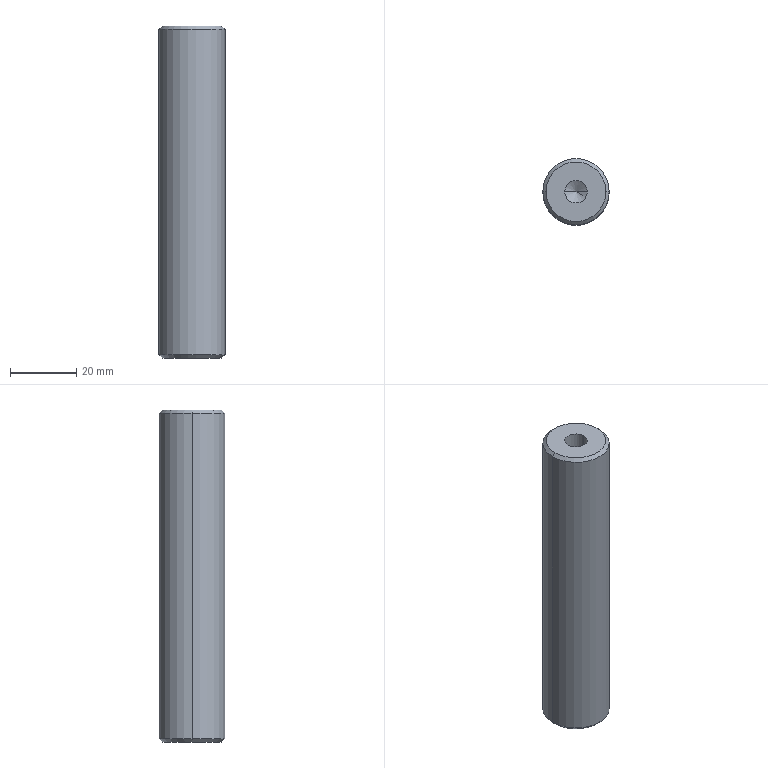Part | SolidWorks | features Chamfer 2, HoleWzd 2, Extrusion 1 | 1 solid | 16 faces | box 20 x 20 x 100 mm | volume 29690 mm3 | cone 8 | cylinder 6 | plane 2 | commonest cylinder face diameters 6.8 x4 20 x2
STEP:
#1=CARTESIAN_POINT('',(3.4,0.,22.25));
#2=VERTEX_POINT('',#1);
#3=CARTESIAN_POINT('',(-3.4,0.,22.25));
#4=VERTEX_POINT('',#3);
#5=CARTESIAN_POINT('',(0.,0.,22.25));
#6=DIRECTION('',(0.,0.,-1.));
#7=DIRECTION('',(-1.,0.,0.));
#8=AXIS2_PLACEMENT_3D('',#5,#6,#7);
#9=CIRCLE('',#8,3.4);
#10=EDGE_CURVE('',#2,#4,#9,.T.);
#11=ORIENTED_EDGE('',*,*,#10,.F.);
#12=CARTESIAN_POINT('',(3.4,0.,0.));
#13=VERTEX_POINT('',#12);
#14=CARTESIAN_POINT('',(3.4,0.,0.));
#15=DIRECTION('',(0.,0.,-1.));
#16=VECTOR('',#15,1000.);
#17=LINE('',#14,#16);
#18=EDGE_CURVE('',#2,#13,#17,.T.);
#19=ORIENTED_EDGE('',*,*,#18,.T.);
#20=CARTESIAN_POINT('',(-3.4,0.,0.));
#21=VERTEX_POINT('',#20);
#22=CARTESIAN_POINT('',(0.,0.,0.));
#23=DIRECTION('',(0.,0.,-1.));
#24=DIRECTION('',(-1.,0.,0.));
#25=AXIS2_PLACEMENT_3D('',#22,#23,#24);
#26=CIRCLE('',#25,3.4);
#27=EDGE_CURVE('',#13,#21,#26,.T.);
#28=ORIENTED_EDGE('',*,*,#27,.T.);
#29=CARTESIAN_POINT('',(-3.4,0.,0.));
#30=DIRECTION('',(0.,0.,-1.));
#31=VECTOR('',#30,1000.);
#32=LINE('',#29,#31);
#33=EDGE_CURVE('',#4,#21,#32,.T.);
#34=ORIENTED_EDGE('',*,*,#33,.F.);
#35=EDGE_LOOP('',(#11,#19,#28,#34));
#36=FACE_OUTER_BOUND('',#35,.T.);
#37=CARTESIAN_POINT('',(0.,0.,0.));
#38=DIRECTION('',(0.,0.,-1.));
#39=DIRECTION('',(-1.,0.,0.));
#40=AXIS2_PLACEMENT_3D('',#37,#38,#39);
#41=CYLINDRICAL_SURFACE('',#40,3.4);
#42=ADVANCED_FACE('',(#36),#41,.F.);
#43=CARTESIAN_POINT('',(0.,0.,24.293));
#44=VERTEX_POINT('',#43);
#45=CARTESIAN_POINT('',(-3.4,0.,22.25));
#46=DIRECTION('',(-0.8572,0.,-0.515));
#47=VECTOR('',#46,1000.);
#48=LINE('',#45,#47);
#49=EDGE_CURVE('',#44,#4,#48,.T.);
#50=ORIENTED_EDGE('',*,*,#49,.F.);
#51=CARTESIAN_POINT('',(3.4,0.,22.25));
#52=DIRECTION('',(0.8572,0.,-0.515));
#53=VECTOR('',#52,1000.);
#54=LINE('',#51,#53);
#55=EDGE_CURVE('',#44,#2,#54,.T.);
#56=ORIENTED_EDGE('',*,*,#55,.T.);
#57=ORIENTED_EDGE('',*,*,#10,.T.);
#58=EDGE_LOOP('',(#50,#56,#57));
#59=FACE_OUTER_BOUND('',#58,.T.);
#60=CARTESIAN_POINT('',(0.,0.,22.25));
#61=DIRECTION('',(0.,0.,-1.));
#62=DIRECTION('',(-1.,0.,0.));
#63=AXIS2_PLACEMENT_3D('',#60,#61,#62);
#64=CONICAL_SURFACE('',#63,3.4,1.03);
#65=ADVANCED_FACE('',(#59),#64,.F.);
#66=CARTESIAN_POINT('',(-9.,0.,0.));
#67=VERTEX_POINT('',#66);
#68=CARTESIAN_POINT('',(9.,0.,0.));
#69=VERTEX_POINT('',#68);
#70=CARTESIAN_POINT('',(0.,0.,0.));
#71=DIRECTION('',(0.,0.,-1.));
#72=DIRECTION('',(1.,0.,0.));
#73=AXIS2_PLACEMENT_3D('',#70,#71,#72);
#74=CIRCLE('',#73,9.);
#75=EDGE_CURVE('',#67,#69,#74,.T.);
#76=ORIENTED_EDGE('',*,*,#75,.F.);
#77=CARTESIAN_POINT('',(-10.,0.,1.));
#78=VERTEX_POINT('',#77);
#79=CARTESIAN_POINT('',(-10.,0.,1.));
#80=DIRECTION('',(-0.7071,0.,0.7071));
#81=VECTOR('',#80,1000.);
#82=LINE('',#79,#81);
#83=EDGE_CURVE('',#67,#78,#82,.T.);
#84=ORIENTED_EDGE('',*,*,#83,.T.);
#85=CARTESIAN_POINT('',(10.,0.,1.));
#86=VERTEX_POINT('',#85);
#87=CARTESIAN_POINT('',(0.,0.,1.));
#88=DIRECTION('',(0.,0.,1.));
#89=DIRECTION('',(1.,0.,0.));
#90=AXIS2_PLACEMENT_3D('',#87,#88,#89);
#91=CIRCLE('',#90,10.);
#92=EDGE_CURVE('',#86,#78,#91,.T.);
#93=ORIENTED_EDGE('',*,*,#92,.F.);
#94=CARTESIAN_POINT('',(10.,0.,1.));
#95=DIRECTION('',(0.7071,0.,0.7071));
#96=VECTOR('',#95,1000.);
#97=LINE('',#94,#96);
#98=EDGE_CURVE('',#69,#86,#97,.T.);
#99=ORIENTED_EDGE('',*,*,#98,.F.);
#100=EDGE_LOOP('',(#76,#84,#93,#99));
#101=FACE_OUTER_BOUND('',#100,.T.);
#102=CARTESIAN_POINT('',(0.,0.,1.));
#103=DIRECTION('',(0.,0.,1.));
#104=DIRECTION('',(1.,0.,0.));
#105=AXIS2_PLACEMENT_3D('',#102,#103,#104);
#106=CONICAL_SURFACE('',#105,10.,0.7854);
#107=ADVANCED_FACE('',(#101),#106,.T.);
#108=CARTESIAN_POINT('',(9.,0.,100.));
#109=VERTEX_POINT('',#108);
#110=CARTESIAN_POINT('',(-9.,0.,100.));
#111=VERTEX_POINT('',#110);
#112=CARTESIAN_POINT('',(0.,0.,100.));
#113=DIRECTION('',(0.,0.,1.));
#114=DIRECTION('',(1.,0.,0.));
#115=AXIS2_PLACEMENT_3D('',#112,#113,#114);
#116=CIRCLE('',#115,9.);
#117=EDGE_CURVE('',#109,#111,#116,.T.);
#118=ORIENTED_EDGE('',*,*,#117,.F.);
#119=CARTESIAN_POINT('',(10.,0.,99.));
#120=VERTEX_POINT('',#119);
#121=CARTESIAN_POINT('',(9.,0.,100.));
#122=DIRECTION('',(0.7071,0.,-0.7071));
#123=VECTOR('',#122,1000.);
#124=LINE('',#121,#123);
#125=EDGE_CURVE('',#109,#120,#124,.T.);
#126=ORIENTED_EDGE('',*,*,#125,.T.);
#127=CARTESIAN_POINT('',(-10.,0.,99.));
#128=VERTEX_POINT('',#127);
#129=CARTESIAN_POINT('',(0.,0.,99.));
#130=DIRECTION('',(0.,0.,-1.));
#131=DIRECTION('',(1.,0.,0.));
#132=AXIS2_PLACEMENT_3D('',#129,#130,#131);
#133=CIRCLE('',#132,10.);
#134=EDGE_CURVE('',#128,#120,#133,.T.);
#135=ORIENTED_EDGE('',*,*,#134,.F.);
#136=CARTESIAN_POINT('',(-9.,0.,100.));
#137=DIRECTION('',(-0.7071,0.,-0.7071));
#138=VECTOR('',#137,1000.);
#139=LINE('',#136,#138);
#140=EDGE_CURVE('',#111,#128,#139,.T.);
#141=ORIENTED_EDGE('',*,*,#140,.F.);
#142=EDGE_LOOP('',(#118,#126,#135,#141));
#143=FACE_OUTER_BOUND('',#142,.T.);
#144=CARTESIAN_POINT('',(0.,0.,100.));
#145=DIRECTION('',(0.,0.,-1.));
#146=DIRECTION('',(-1.,0.,0.));
#147=AXIS2_PLACEMENT_3D('',#144,#145,#146);
#148=CONICAL_SURFACE('',#147,9.,0.7854);
#149=ADVANCED_FACE('',(#143),#148,.T.);
#150=CARTESIAN_POINT('',(-3.4,0.,77.75));
#151=VERTEX_POINT('',#150);
#152=CARTESIAN_POINT('',(3.4,0.,77.75));
#153=VERTEX_POINT('',#152);
#154=CARTESIAN_POINT('',(0.,0.,77.75));
#155=DIRECTION('',(0.,0.,1.));
#156=DIRECTION('',(1.,0.,0.));
#157=AXIS2_PLACEMENT_3D('',#154,#155,#156);
#158=CIRCLE('',#157,3.4);
#159=EDGE_CURVE('',#151,#153,#158,.T.);
#160=ORIENTED_EDGE('',*,*,#159,.F.);
#161=CARTESIAN_POINT('',(-3.4,0.,100.));
#162=VERTEX_POINT('',#161);
#163=CARTESIAN_POINT('',(-3.4,0.,100.));
#164=DIRECTION('',(0.,0.,1.));
#165=VECTOR('',#164,1000.);
#166=LINE('',#163,#165);
#167=EDGE_CURVE('',#151,#162,#166,.T.);
#168=ORIENTED_EDGE('',*,*,#167,.T.);
#169=CARTESIAN_POINT('',(3.4,0.,100.));
#170=VERTEX_POINT('',#169);
#171=CARTESIAN_POINT('',(0.,0.,100.));
#172=DIRECTION('',(0.,0.,1.));
#173=DIRECTION('',(1.,0.,0.));
#174=AXIS2_PLACEMENT_3D('',#171,#172,#173);
#175=CIRCLE('',#174,3.4);
#176=EDGE_CURVE('',#162,#170,#175,.T.);
#177=ORIENTED_EDGE('',*,*,#176,.T.);
#178=CARTESIAN_POINT('',(3.4,0.,100.));
#179=DIRECTION('',(0.,0.,1.));
#180=VECTOR('',#179,1000.);
#181=LINE('',#178,#180);
#182=EDGE_CURVE('',#153,#170,#181,.T.);
#183=ORIENTED_EDGE('',*,*,#182,.F.);
#184=EDGE_LOOP('',(#160,#168,#177,#183));
#185=FACE_OUTER_BOUND('',#184,.T.);
#186=CARTESIAN_POINT('',(0.,0.,100.));
#187=DIRECTION('',(0.,0.,1.));
#188=DIRECTION('',(1.,0.,0.));
#189=AXIS2_PLACEMENT_3D('',#186,#187,#188);
#190=CYLINDRICAL_SURFACE('',#189,3.4);
#191=ADVANCED_FACE('',(#185),#190,.F.);
#192=CARTESIAN_POINT('',(0.,0.,75.707));
#193=VERTEX_POINT('',#192);
#194=CARTESIAN_POINT('',(3.4,0.,77.75));
#195=DIRECTION('',(0.8572,0.,0.515));
#196=VECTOR('',#195,1000.);
#197=LINE('',#194,#196);
#198=EDGE_CURVE('',#193,#153,#197,.T.);
#199=ORIENTED_EDGE('',*,*,#198,.F.);
#200=CARTESIAN_POINT('',(-3.4,0.,77.75));
#201=DIRECTION('',(-0.8572,0.,0.515));
#202=VECTOR('',#201,1000.);
#203=LINE('',#200,#202);
#204=EDGE_CURVE('',#193,#151,#203,.T.);
#205=ORIENTED_EDGE('',*,*,#204,.T.);
#206=ORIENTED_EDGE('',*,*,#159,.T.);
#207=EDGE_LOOP('',(#199,#205,#206));
#208=FACE_OUTER_BOUND('',#207,.T.);
#209=CARTESIAN_POINT('',(0.,0.,77.75));
#210=DIRECTION('',(0.,0.,1.));
#211=DIRECTION('',(1.,0.,0.));
#212=AXIS2_PLACEMENT_3D('',#209,#210,#211);
#213=CONICAL_SURFACE('',#212,3.4,1.03);
#214=ADVANCED_FACE('',(#208),#213,.F.);
#215=ORIENTED_EDGE('',*,*,#134,.T.);
#216=CARTESIAN_POINT('',(10.,0.,100.));
#217=DIRECTION('',(0.,0.,-1.));
#218=VECTOR('',#217,1000.);
#219=LINE('',#216,#218);
#220=EDGE_CURVE('',#120,#86,#219,.T.);
#221=ORIENTED_EDGE('',*,*,#220,.T.);
#222=ORIENTED_EDGE('',*,*,#92,.T.);
#223=CARTESIAN_POINT('',(-10.,0.,100.));
#224=DIRECTION('',(0.,0.,-1.));
#225=VECTOR('',#224,1000.);
#226=LINE('',#223,#225);
#227=EDGE_CURVE('',#128,#78,#226,.T.);
#228=ORIENTED_EDGE('',*,*,#227,.F.);
#229=EDGE_LOOP('',(#215,#221,#222,#228));
#230=FACE_OUTER_BOUND('',#229,.T.);
#231=CARTESIAN_POINT('',(0.,0.,100.));
#232=DIRECTION('',(0.,0.,-1.));
#233=DIRECTION('',(-1.,0.,0.));
#234=AXIS2_PLACEMENT_3D('',#231,#232,#233);
#235=CYLINDRICAL_SURFACE('',#234,10.);
#236=ADVANCED_FACE('',(#230),#235,.T.);
#237=ORIENTED_EDGE('',*,*,#220,.F.);
#238=CARTESIAN_POINT('',(0.,0.,99.));
#239=DIRECTION('',(0.,0.,-1.));
#240=DIRECTION('',(1.,0.,0.));
#241=AXIS2_PLACEMENT_3D('',#238,#239,#240);
#242=CIRCLE('',#241,10.);
#243=EDGE_CURVE('',#120,#128,#242,.T.);
#244=ORIENTED_EDGE('',*,*,#243,.T.);
#245=ORIENTED_EDGE('',*,*,#227,.T.);
#246=CARTESIAN_POINT('',(0.,0.,1.));
#247=DIRECTION('',(0.,0.,1.));
#248=DIRECTION('',(1.,0.,0.));
#249=AXIS2_PLACEMENT_3D('',#246,#247,#248);
#250=CIRCLE('',#249,10.);
#251=EDGE_CURVE('',#78,#86,#250,.T.);
#252=ORIENTED_EDGE('',*,*,#251,.T.);
#253=EDGE_LOOP('',(#237,#244,#245,#252));
#254=FACE_OUTER_BOUND('',#253,.T.);
#255=CARTESIAN_POINT('',(0.,0.,100.));
#256=DIRECTION('',(0.,0.,-1.));
#257=DIRECTION('',(-1.,0.,0.));
#258=AXIS2_PLACEMENT_3D('',#255,#256,#257);
#259=CYLINDRICAL_SURFACE('',#258,10.);
#260=ADVANCED_FACE('',(#254),#259,.T.);
#261=CARTESIAN_POINT('',(0.,0.,100.));
#262=DIRECTION('',(0.,0.,1.));
#263=DIRECTION('',(1.,0.,0.));
#264=AXIS2_PLACEMENT_3D('',#261,#262,#263);
#265=CIRCLE('',#264,9.);
#266=EDGE_CURVE('',#111,#109,#265,.T.);
#267=ORIENTED_EDGE('',*,*,#266,.T.);
#268=ORIENTED_EDGE('',*,*,#117,.T.);
#269=EDGE_LOOP('',(#267,#268));
#270=FACE_OUTER_BOUND('',#269,.T.);
#271=CARTESIAN_POINT('',(0.,0.,100.));
#272=DIRECTION('',(0.,0.,1.));
#273=DIRECTION('',(1.,0.,0.));
#274=AXIS2_PLACEMENT_3D('',#271,#272,#273);
#275=CIRCLE('',#274,3.4);
#276=EDGE_CURVE('',#170,#162,#275,.T.);
#277=ORIENTED_EDGE('',*,*,#276,.F.);
#278=ORIENTED_EDGE('',*,*,#176,.F.);
#279=EDGE_LOOP('',(#277,#278));
#280=FACE_BOUND('',#279,.T.);
#281=CARTESIAN_POINT('',(0.,0.,100.));
#282=DIRECTION('',(0.,0.,1.));
#283=DIRECTION('',(1.,0.,0.));
#284=AXIS2_PLACEMENT_3D('',#281,#282,#283);
#285=PLANE('',#284);
#286=ADVANCED_FACE('',(#270,#280),#285,.T.);
#287=CARTESIAN_POINT('',(0.,0.,0.));
#288=DIRECTION('',(0.,0.,-1.));
#289=DIRECTION('',(-1.,0.,0.));
#290=AXIS2_PLACEMENT_3D('',#287,#288,#289);
#291=CIRCLE('',#290,3.4);
#292=EDGE_CURVE('',#21,#13,#291,.T.);
#293=ORIENTED_EDGE('',*,*,#292,.F.);
#294=ORIENTED_EDGE('',*,*,#27,.F.);
#295=EDGE_LOOP('',(#293,#294));
#296=FACE_BOUND('',#295,.T.);
#297=CARTESIAN_POINT('',(0.,0.,0.));
#298=DIRECTION('',(0.,0.,-1.));
#299=DIRECTION('',(1.,0.,0.));
#300=AXIS2_PLACEMENT_3D('',#297,#298,#299);
#301=CIRCLE('',#300,9.);
#302=EDGE_CURVE('',#69,#67,#301,.T.);
#303=ORIENTED_EDGE('',*,*,#302,.T.);
#304=ORIENTED_EDGE('',*,*,#75,.T.);
#305=EDGE_LOOP('',(#303,#304));
#306=FACE_OUTER_BOUND('',#305,.T.);
#307=CARTESIAN_POINT('',(0.,0.,0.));
#308=DIRECTION('',(0.,0.,1.));
#309=DIRECTION('',(1.,0.,0.));
#310=AXIS2_PLACEMENT_3D('',#307,#308,#309);
#311=PLANE('',#310);
#312=ADVANCED_FACE('',(#296,#306),#311,.F.);
#313=ORIENTED_EDGE('',*,*,#204,.F.);
#314=ORIENTED_EDGE('',*,*,#198,.T.);
#315=CARTESIAN_POINT('',(0.,0.,77.75));
#316=DIRECTION('',(0.,0.,1.));
#317=DIRECTION('',(1.,0.,0.));
#318=AXIS2_PLACEMENT_3D('',#315,#316,#317);
#319=CIRCLE('',#318,3.4);
#320=EDGE_CURVE('',#153,#151,#319,.T.);
#321=ORIENTED_EDGE('',*,*,#320,.T.);
#322=EDGE_LOOP('',(#313,#314,#321));
#323=FACE_OUTER_BOUND('',#322,.T.);
#324=CARTESIAN_POINT('',(0.,0.,77.75));
#325=DIRECTION('',(0.,0.,1.));
#326=DIRECTION('',(1.,0.,0.));
#327=AXIS2_PLACEMENT_3D('',#324,#325,#326);
#328=CONICAL_SURFACE('',#327,3.4,1.03);
#329=ADVANCED_FACE('',(#323),#328,.F.);
#330=ORIENTED_EDGE('',*,*,#167,.F.);
#331=ORIENTED_EDGE('',*,*,#320,.F.);
#332=ORIENTED_EDGE('',*,*,#182,.T.);
#333=ORIENTED_EDGE('',*,*,#276,.T.);
#334=EDGE_LOOP('',(#330,#331,#332,#333));
#335=FACE_OUTER_BOUND('',#334,.T.);
#336=CARTESIAN_POINT('',(0.,0.,100.));
#337=DIRECTION('',(0.,0.,1.));
#338=DIRECTION('',(1.,0.,0.));
#339=AXIS2_PLACEMENT_3D('',#336,#337,#338);
#340=CYLINDRICAL_SURFACE('',#339,3.4);
#341=ADVANCED_FACE('',(#335),#340,.F.);
#342=ORIENTED_EDGE('',*,*,#125,.F.);
#343=ORIENTED_EDGE('',*,*,#266,.F.);
#344=ORIENTED_EDGE('',*,*,#140,.T.);
#345=ORIENTED_EDGE('',*,*,#243,.F.);
#346=EDGE_LOOP('',(#342,#343,#344,#345));
#347=FACE_OUTER_BOUND('',#346,.T.);
#348=CARTESIAN_POINT('',(0.,0.,100.));
#349=DIRECTION('',(0.,0.,-1.));
#350=DIRECTION('',(-1.,0.,0.));
#351=AXIS2_PLACEMENT_3D('',#348,#349,#350);
#352=CONICAL_SURFACE('',#351,9.,0.7854);
#353=ADVANCED_FACE('',(#347),#352,.T.);
#354=ORIENTED_EDGE('',*,*,#83,.F.);
#355=ORIENTED_EDGE('',*,*,#302,.F.);
#356=ORIENTED_EDGE('',*,*,#98,.T.);
#357=ORIENTED_EDGE('',*,*,#251,.F.);
#358=EDGE_LOOP('',(#354,#355,#356,#357));
#359=FACE_OUTER_BOUND('',#358,.T.);
#360=CARTESIAN_POINT('',(0.,0.,1.));
#361=DIRECTION('',(0.,0.,1.));
#362=DIRECTION('',(1.,0.,0.));
#363=AXIS2_PLACEMENT_3D('',#360,#361,#362);
#364=CONICAL_SURFACE('',#363,10.,0.7854);
#365=ADVANCED_FACE('',(#359),#364,.T.);
#366=ORIENTED_EDGE('',*,*,#55,.F.);
#367=ORIENTED_EDGE('',*,*,#49,.T.);
#368=CARTESIAN_POINT('',(0.,0.,22.25));
#369=DIRECTION('',(0.,0.,-1.));
#370=DIRECTION('',(-1.,0.,0.));
#371=AXIS2_PLACEMENT_3D('',#368,#369,#370);
#372=CIRCLE('',#371,3.4);
#373=EDGE_CURVE('',#4,#2,#372,.T.);
#374=ORIENTED_EDGE('',*,*,#373,.T.);
#375=EDGE_LOOP('',(#366,#367,#374));
#376=FACE_OUTER_BOUND('',#375,.T.);
#377=CARTESIAN_POINT('',(0.,0.,22.25));
#378=DIRECTION('',(0.,0.,-1.));
#379=DIRECTION('',(-1.,0.,0.));
#380=AXIS2_PLACEMENT_3D('',#377,#378,#379);
#381=CONICAL_SURFACE('',#380,3.4,1.03);
#382=ADVANCED_FACE('',(#376),#381,.F.);
#383=ORIENTED_EDGE('',*,*,#18,.F.);
#384=ORIENTED_EDGE('',*,*,#373,.F.);
#385=ORIENTED_EDGE('',*,*,#33,.T.);
#386=ORIENTED_EDGE('',*,*,#292,.T.);
#387=EDGE_LOOP('',(#383,#384,#385,#386));
#388=FACE_OUTER_BOUND('',#387,.T.);
#389=CARTESIAN_POINT('',(0.,0.,0.));
#390=DIRECTION('',(0.,0.,-1.));
#391=DIRECTION('',(-1.,0.,0.));
#392=AXIS2_PLACEMENT_3D('',#389,#390,#391);
#393=CYLINDRICAL_SURFACE('',#392,3.4);
#394=ADVANCED_FACE('',(#388),#393,.F.);
#395=CLOSED_SHELL('',(#42,#65,#107,#149,#191,#214,#236,#260,#286,#312,#329,#341,#353,#365,#382,#394));
#396=MANIFOLD_SOLID_BREP('',#395);
#397=CARTESIAN_POINT('',(0.,0.,0.));
#398=DIRECTION('',(0.,0.,1.));
#399=DIRECTION('',(1.,0.,0.));
#400=AXIS2_PLACEMENT_3D('',#397,#398,#399);
#401=(LENGTH_UNIT()NAMED_UNIT(*)SI_UNIT(.MILLI.,.METRE.));
#402=UNCERTAINTY_MEASURE_WITH_UNIT(LENGTH_MEASURE(0.00001),#401,'','');
#403=(NAMED_UNIT(*)PLANE_ANGLE_UNIT()SI_UNIT($,.RADIAN.));
#404=(NAMED_UNIT(*)SI_UNIT($,.STERADIAN.)SOLID_ANGLE_UNIT());
#405=(GEOMETRIC_REPRESENTATION_CONTEXT(3)GLOBAL_UNCERTAINTY_ASSIGNED_CONTEXT((#402))GLOBAL_UNIT_ASSIGNED_CONTEXT((#401,#403,#404))REPRESENTATION_CONTEXT('',''));
#406=ADVANCED_BREP_SHAPE_REPRESENTATION('',(#396,#400),#405);